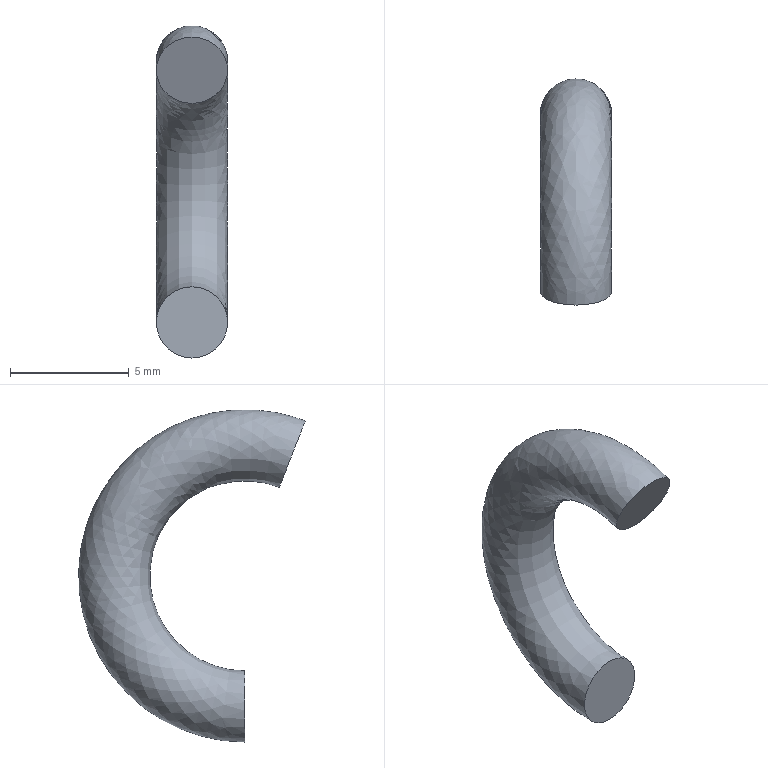Part | NX | features solid 2 | 1 solid | 3 faces | box 3 x 9.543 x 13.998 mm | volume 136.616 mm3 | plane 2 | spline 1
STEP:
#1=CARTESIAN_POINT('',(-1551.,413.545,19.726));
#2=VERTEX_POINT('',#1);
#3=CARTESIAN_POINT('',(-1551.,413.,21.123));
#4=DIRECTION('',(0.,-0.9315,-0.3636));
#5=DIRECTION('',(0.,0.3636,-0.9315));
#6=AXIS2_PLACEMENT_3D('',#3,#4,#5);
#7=CIRCLE('',#6,1.5);
#8=EDGE_CURVE('',#2,#2,#7,.T.);
#9=ORIENTED_EDGE('',*,*,#8,.T.);
#10=EDGE_LOOP('',(#9));
#11=FACE_BOUND('',#10,.T.);
#12=CARTESIAN_POINT('',(-1551.,413.,21.123));
#13=DIRECTION('',(0.,-0.9315,-0.3636));
#14=DIRECTION('',(0.,0.3636,-0.9315));
#15=AXIS2_PLACEMENT_3D('',#12,#13,#14);
#16=PLANE('',#15);
#17=ADVANCED_FACE('',(#11),#16,.T.);
#18=CARTESIAN_POINT('',(-1551.,415.,9.));
#19=VERTEX_POINT('',#18);
#20=CARTESIAN_POINT('',(-1551.,415.,10.5));
#21=DIRECTION('',(0.,-1.,0.));
#22=DIRECTION('',(0.,0.,-1.));
#23=AXIS2_PLACEMENT_3D('',#20,#21,#22);
#24=CIRCLE('',#23,1.5);
#25=EDGE_CURVE('',#19,#19,#24,.T.);
#26=ORIENTED_EDGE('',*,*,#25,.T.);
#27=EDGE_LOOP('',(#26));
#28=FACE_BOUND('',#27,.T.);
#29=CARTESIAN_POINT('',(-1551.,415.,10.5));
#30=DIRECTION('',(0.,-1.,0.));
#31=DIRECTION('',(0.,0.,-1.));
#32=AXIS2_PLACEMENT_3D('',#29,#30,#31);
#33=PLANE('',#32);
#34=ADVANCED_FACE('',(#28),#33,.T.);
#35=ORIENTED_EDGE('',*,*,#25,.F.);
#36=EDGE_LOOP('',(#35));
#37=FACE_BOUND('',#36,.T.);
#38=ORIENTED_EDGE('',*,*,#8,.F.);
#39=EDGE_LOOP('',(#38));
#40=FACE_BOUND('',#39,.T.);
#41=CARTESIAN_POINT('',(-1549.5,415.,9.97));
#42=CARTESIAN_POINT('',(-1549.5,416.255,9.958));
#43=CARTESIAN_POINT('',(-1549.5,417.618,10.391));
#44=CARTESIAN_POINT('',(-1549.5,419.793,12.094));
#45=CARTESIAN_POINT('',(-1549.5,420.5,13.222));
#46=CARTESIAN_POINT('',(-1549.5,421.165,15.703));
#47=CARTESIAN_POINT('',(-1549.5,421.079,17.179));
#48=CARTESIAN_POINT('',(-1549.5,420.163,19.234));
#49=CARTESIAN_POINT('',(-1549.5,419.645,19.935));
#50=CARTESIAN_POINT('',(-1549.5,418.39,21.062));
#51=CARTESIAN_POINT('',(-1549.5,416.38,22.219));
#52=CARTESIAN_POINT('',(-1549.5,413.962,22.092));
#53=CARTESIAN_POINT('',(-1549.5,412.807,21.617));
#54=CARTESIAN_POINT('',(-1549.5,415.,11.03));
#55=CARTESIAN_POINT('',(-1549.5,416.034,11.02));
#56=CARTESIAN_POINT('',(-1549.5,417.157,11.378));
#57=CARTESIAN_POINT('',(-1549.5,418.95,12.781));
#58=CARTESIAN_POINT('',(-1549.5,419.533,13.711));
#59=CARTESIAN_POINT('',(-1549.5,420.081,15.755));
#60=CARTESIAN_POINT('',(-1549.5,420.01,16.971));
#61=CARTESIAN_POINT('',(-1549.5,419.255,18.665));
#62=CARTESIAN_POINT('',(-1549.5,418.828,19.243));
#63=CARTESIAN_POINT('',(-1549.5,417.794,20.172));
#64=CARTESIAN_POINT('',(-1549.5,416.138,21.125));
#65=CARTESIAN_POINT('',(-1549.5,414.144,21.02));
#66=CARTESIAN_POINT('',(-1549.5,413.193,20.629));
#67=CARTESIAN_POINT('',(-1549.765,415.,11.735));
#68=CARTESIAN_POINT('',(-1549.765,415.888,11.726));
#69=CARTESIAN_POINT('',(-1549.765,416.851,12.033));
#70=CARTESIAN_POINT('',(-1549.765,418.39,13.237));
#71=CARTESIAN_POINT('',(-1549.765,418.89,14.035));
#72=CARTESIAN_POINT('',(-1549.765,419.36,15.79));
#73=CARTESIAN_POINT('',(-1549.765,419.3,16.834));
#74=CARTESIAN_POINT('',(-1549.765,418.652,18.288));
#75=CARTESIAN_POINT('',(-1549.765,418.285,18.783));
#76=CARTESIAN_POINT('',(-1549.765,417.398,19.58));
#77=CARTESIAN_POINT('',(-1549.765,415.976,20.398));
#78=CARTESIAN_POINT('',(-1549.765,414.266,20.308));
#79=CARTESIAN_POINT('',(-1549.765,413.449,19.973));
#80=CARTESIAN_POINT('',(-1550.47,415.,12.));
#81=CARTESIAN_POINT('',(-1550.47,415.833,11.992));
#82=CARTESIAN_POINT('',(-1550.47,416.736,12.28));
#83=CARTESIAN_POINT('',(-1550.47,418.179,13.409));
#84=CARTESIAN_POINT('',(-1550.47,418.648,14.158));
#85=CARTESIAN_POINT('',(-1550.47,419.089,15.803));
#86=CARTESIAN_POINT('',(-1550.47,419.032,16.782));
#87=CARTESIAN_POINT('',(-1550.47,418.425,18.145));
#88=CARTESIAN_POINT('',(-1550.47,418.081,18.61));
#89=CARTESIAN_POINT('',(-1550.47,417.249,19.358));
#90=CARTESIAN_POINT('',(-1550.47,415.916,20.125));
#91=CARTESIAN_POINT('',(-1550.47,414.311,20.041));
#92=CARTESIAN_POINT('',(-1550.47,413.545,19.726));
#93=CARTESIAN_POINT('',(-1551.53,415.,12.));
#94=CARTESIAN_POINT('',(-1551.53,415.833,11.992));
#95=CARTESIAN_POINT('',(-1551.53,416.736,12.28));
#96=CARTESIAN_POINT('',(-1551.53,418.179,13.409));
#97=CARTESIAN_POINT('',(-1551.53,418.648,14.158));
#98=CARTESIAN_POINT('',(-1551.53,419.089,15.803));
#99=CARTESIAN_POINT('',(-1551.53,419.032,16.782));
#100=CARTESIAN_POINT('',(-1551.53,418.425,18.145));
#101=CARTESIAN_POINT('',(-1551.53,418.081,18.61));
#102=CARTESIAN_POINT('',(-1551.53,417.249,19.358));
#103=CARTESIAN_POINT('',(-1551.53,415.916,20.125));
#104=CARTESIAN_POINT('',(-1551.53,414.311,20.041));
#105=CARTESIAN_POINT('',(-1551.53,413.545,19.726));
#106=CARTESIAN_POINT('',(-1552.235,415.,11.735));
#107=CARTESIAN_POINT('',(-1552.235,415.888,11.726));
#108=CARTESIAN_POINT('',(-1552.235,416.851,12.033));
#109=CARTESIAN_POINT('',(-1552.235,418.39,13.237));
#110=CARTESIAN_POINT('',(-1552.235,418.89,14.035));
#111=CARTESIAN_POINT('',(-1552.235,419.36,15.79));
#112=CARTESIAN_POINT('',(-1552.235,419.3,16.834));
#113=CARTESIAN_POINT('',(-1552.235,418.652,18.288));
#114=CARTESIAN_POINT('',(-1552.235,418.285,18.783));
#115=CARTESIAN_POINT('',(-1552.235,417.398,19.58));
#116=CARTESIAN_POINT('',(-1552.235,415.976,20.398));
#117=CARTESIAN_POINT('',(-1552.235,414.266,20.308));
#118=CARTESIAN_POINT('',(-1552.235,413.449,19.973));
#119=CARTESIAN_POINT('',(-1552.5,415.,11.03));
#120=CARTESIAN_POINT('',(-1552.5,416.034,11.02));
#121=CARTESIAN_POINT('',(-1552.5,417.157,11.378));
#122=CARTESIAN_POINT('',(-1552.5,418.95,12.781));
#123=CARTESIAN_POINT('',(-1552.5,419.533,13.711));
#124=CARTESIAN_POINT('',(-1552.5,420.081,15.755));
#125=CARTESIAN_POINT('',(-1552.5,420.01,16.971));
#126=CARTESIAN_POINT('',(-1552.5,419.255,18.665));
#127=CARTESIAN_POINT('',(-1552.5,418.828,19.243));
#128=CARTESIAN_POINT('',(-1552.5,417.794,20.172));
#129=CARTESIAN_POINT('',(-1552.5,416.138,21.125));
#130=CARTESIAN_POINT('',(-1552.5,414.144,21.02));
#131=CARTESIAN_POINT('',(-1552.5,413.193,20.629));
#132=CARTESIAN_POINT('',(-1552.5,415.,9.97));
#133=CARTESIAN_POINT('',(-1552.5,416.255,9.958));
#134=CARTESIAN_POINT('',(-1552.5,417.618,10.391));
#135=CARTESIAN_POINT('',(-1552.5,419.793,12.094));
#136=CARTESIAN_POINT('',(-1552.5,420.5,13.222));
#137=CARTESIAN_POINT('',(-1552.5,421.165,15.703));
#138=CARTESIAN_POINT('',(-1552.5,421.079,17.179));
#139=CARTESIAN_POINT('',(-1552.5,420.163,19.234));
#140=CARTESIAN_POINT('',(-1552.5,419.645,19.935));
#141=CARTESIAN_POINT('',(-1552.5,418.39,21.062));
#142=CARTESIAN_POINT('',(-1552.5,416.38,22.219));
#143=CARTESIAN_POINT('',(-1552.5,413.962,22.092));
#144=CARTESIAN_POINT('',(-1552.5,412.807,21.617));
#145=CARTESIAN_POINT('',(-1552.235,415.,9.265));
#146=CARTESIAN_POINT('',(-1552.235,416.402,9.252));
#147=CARTESIAN_POINT('',(-1552.235,417.923,9.736));
#148=CARTESIAN_POINT('',(-1552.235,420.353,11.638));
#149=CARTESIAN_POINT('',(-1552.235,421.143,12.898));
#150=CARTESIAN_POINT('',(-1552.235,421.885,15.668));
#151=CARTESIAN_POINT('',(-1552.235,421.789,17.317));
#152=CARTESIAN_POINT('',(-1552.235,420.767,19.612));
#153=CARTESIAN_POINT('',(-1552.235,420.188,20.395));
#154=CARTESIAN_POINT('',(-1552.235,418.786,21.653));
#155=CARTESIAN_POINT('',(-1552.235,416.542,22.945));
#156=CARTESIAN_POINT('',(-1552.235,413.84,22.803));
#157=CARTESIAN_POINT('',(-1552.235,412.551,22.274));
#158=CARTESIAN_POINT('',(-1551.53,415.,9.));
#159=CARTESIAN_POINT('',(-1551.53,416.457,8.986));
#160=CARTESIAN_POINT('',(-1551.53,418.038,9.49));
#161=CARTESIAN_POINT('',(-1551.53,420.564,11.466));
#162=CARTESIAN_POINT('',(-1551.53,421.384,12.776));
#163=CARTESIAN_POINT('',(-1551.53,422.156,15.655));
#164=CARTESIAN_POINT('',(-1551.53,422.056,17.368));
#165=CARTESIAN_POINT('',(-1551.53,420.994,19.754));
#166=CARTESIAN_POINT('',(-1551.53,420.392,20.568));
#167=CARTESIAN_POINT('',(-1551.53,418.935,21.876));
#168=CARTESIAN_POINT('',(-1551.53,416.602,23.218));
#169=CARTESIAN_POINT('',(-1551.53,413.795,23.071));
#170=CARTESIAN_POINT('',(-1551.53,412.455,22.521));
#171=CARTESIAN_POINT('',(-1550.47,415.,9.));
#172=CARTESIAN_POINT('',(-1550.47,416.457,8.986));
#173=CARTESIAN_POINT('',(-1550.47,418.038,9.49));
#174=CARTESIAN_POINT('',(-1550.47,420.564,11.466));
#175=CARTESIAN_POINT('',(-1550.47,421.384,12.776));
#176=CARTESIAN_POINT('',(-1550.47,422.156,15.655));
#177=CARTESIAN_POINT('',(-1550.47,422.056,17.368));
#178=CARTESIAN_POINT('',(-1550.47,420.994,19.754));
#179=CARTESIAN_POINT('',(-1550.47,420.392,20.568));
#180=CARTESIAN_POINT('',(-1550.47,418.935,21.876));
#181=CARTESIAN_POINT('',(-1550.47,416.602,23.218));
#182=CARTESIAN_POINT('',(-1550.47,413.795,23.071));
#183=CARTESIAN_POINT('',(-1550.47,412.455,22.521));
#184=CARTESIAN_POINT('',(-1549.765,415.,9.265));
#185=CARTESIAN_POINT('',(-1549.765,416.402,9.252));
#186=CARTESIAN_POINT('',(-1549.765,417.923,9.736));
#187=CARTESIAN_POINT('',(-1549.765,420.353,11.638));
#188=CARTESIAN_POINT('',(-1549.765,421.143,12.898));
#189=CARTESIAN_POINT('',(-1549.765,421.885,15.668));
#190=CARTESIAN_POINT('',(-1549.765,421.789,17.317));
#191=CARTESIAN_POINT('',(-1549.765,420.767,19.612));
#192=CARTESIAN_POINT('',(-1549.765,420.188,20.395));
#193=CARTESIAN_POINT('',(-1549.765,418.786,21.653));
#194=CARTESIAN_POINT('',(-1549.765,416.542,22.945));
#195=CARTESIAN_POINT('',(-1549.765,413.84,22.803));
#196=CARTESIAN_POINT('',(-1549.765,412.551,22.274));
#197=CARTESIAN_POINT('',(-1549.5,415.,9.97));
#198=CARTESIAN_POINT('',(-1549.5,416.255,9.958));
#199=CARTESIAN_POINT('',(-1549.5,417.618,10.391));
#200=CARTESIAN_POINT('',(-1549.5,419.793,12.094));
#201=CARTESIAN_POINT('',(-1549.5,420.5,13.222));
#202=CARTESIAN_POINT('',(-1549.5,421.165,15.703));
#203=CARTESIAN_POINT('',(-1549.5,421.079,17.179));
#204=CARTESIAN_POINT('',(-1549.5,420.163,19.234));
#205=CARTESIAN_POINT('',(-1549.5,419.645,19.935));
#206=CARTESIAN_POINT('',(-1549.5,418.39,21.062));
#207=CARTESIAN_POINT('',(-1549.5,416.38,22.219));
#208=CARTESIAN_POINT('',(-1549.5,413.962,22.092));
#209=CARTESIAN_POINT('',(-1549.5,412.807,21.617));
#210=CARTESIAN_POINT('',(-1549.5,415.,11.03));
#211=CARTESIAN_POINT('',(-1549.5,416.034,11.02));
#212=CARTESIAN_POINT('',(-1549.5,417.157,11.378));
#213=CARTESIAN_POINT('',(-1549.5,418.95,12.781));
#214=CARTESIAN_POINT('',(-1549.5,419.533,13.711));
#215=CARTESIAN_POINT('',(-1549.5,420.081,15.755));
#216=CARTESIAN_POINT('',(-1549.5,420.01,16.971));
#217=CARTESIAN_POINT('',(-1549.5,419.255,18.665));
#218=CARTESIAN_POINT('',(-1549.5,418.828,19.243));
#219=CARTESIAN_POINT('',(-1549.5,417.794,20.172));
#220=CARTESIAN_POINT('',(-1549.5,416.138,21.125));
#221=CARTESIAN_POINT('',(-1549.5,414.144,21.02));
#222=CARTESIAN_POINT('',(-1549.5,413.193,20.629));
#223=(BOUNDED_SURFACE()B_SPLINE_SURFACE(4,3,((#41,#42,#43,#44,#45,#46,#47,#48,#49,#50,#51,#52,#53),(#54,#55,#56,#57,#58,#59,#60,#61,#62,#63,#64,#65,#66),(#67,#68,#69,#70,#71,#72,#73,#74,#75,#76,#77,#78,#79),(#80,#81,#82,#83,#84,#85,#86,#87,#88,#89,#90,#91,#92),(#93,#94,#95,#96,#97,#98,#99,#100,#101,#102,#103,#104,#105),(#106,#107,#108,#109,#110,#111,#112,#113,#114,#115,#116,#117,#118),(#119,#120,#121,#122,#123,#124,#125,#126,#127,#128,#129,#130,#131),(#132,#133,#134,#135,#136,#137,#138,#139,#140,#141,#142,#143,#144),(#145,#146,#147,#148,#149,#150,#151,#152,#153,#154,#155,#156,#157),(#158,#159,#160,#161,#162,#163,#164,#165,#166,#167,#168,#169,#170),(#171,#172,#173,#174,#175,#176,#177,#178,#179,#180,#181,#182,#183),(#184,#185,#186,#187,#188,#189,#190,#191,#192,#193,#194,#195,#196),(#197,#198,#199,#200,#201,#202,#203,#204,#205,#206,#207,#208,#209),(#210,#211,#212,#213,#214,#215,#216,#217,#218,#219,#220,#221,#222)),.UNSPECIFIED.,.T.,.F.,.F.)B_SPLINE_SURFACE_WITH_KNOTS((2,3,3,3,3,3,2),(4,2,2,2,2,1,4),(-0.25,0.,0.25,0.5,0.75,1.,1.25),(0.,0.1875,0.375,0.5625,0.6875,0.8125,1.),.UNSPECIFIED.)GEOMETRIC_REPRESENTATION_ITEM()RATIONAL_B_SPLINE_SURFACE(((1.017,1.017,1.017,1.017,1.017,1.017,1.017,1.017,1.017,1.017,1.017,1.017,1.017),(1.017,1.017,1.017,1.017,1.017,1.017,1.017,1.017,1.017,1.017,1.017,1.017,1.017),(0.9585,0.9585,0.9585,0.9585,0.9585,0.9585,0.9585,0.9585,0.9585,0.9585,0.9585,0.9585,0.9585),(1.017,1.017,1.017,1.017,1.017,1.017,1.017,1.017,1.017,1.017,1.017,1.017,1.017),(1.017,1.017,1.017,1.017,1.017,1.017,1.017,1.017,1.017,1.017,1.017,1.017,1.017),(0.9585,0.9585,0.9585,0.9585,0.9585,0.9585,0.9585,0.9585,0.9585,0.9585,0.9585,0.9585,0.9585),(1.017,1.017,1.017,1.017,1.017,1.017,1.017,1.017,1.017,1.017,1.017,1.017,1.017),(1.017,1.017,1.017,1.017,1.017,1.017,1.017,1.017,1.017,1.017,1.017,1.017,1.017),(0.9585,0.9585,0.9585,0.9585,0.9585,0.9585,0.9585,0.9585,0.9585,0.9585,0.9585,0.9585,0.9585),(1.017,1.017,1.017,1.017,1.017,1.017,1.017,1.017,1.017,1.017,1.017,1.017,1.017),(1.017,1.017,1.017,1.017,1.017,1.017,1.017,1.017,1.017,1.017,1.017,1.017,1.017),(0.9585,0.9585,0.9585,0.9585,0.9585,0.9585,0.9585,0.9585,0.9585,0.9585,0.9585,0.9585,0.9585),(1.017,1.017,1.017,1.017,1.017,1.017,1.017,1.017,1.017,1.017,1.017,1.017,1.017),(1.017,1.017,1.017,1.017,1.017,1.017,1.017,1.017,1.017,1.017,1.017,1.017,1.017)))REPRESENTATION_ITEM('')SURFACE());
#224=ADVANCED_FACE('',(#37,#40),#223,.F.);
#225=CLOSED_SHELL('',(#17,#34,#224));
#226=MANIFOLD_SOLID_BREP('',#225);
#227=(LENGTH_UNIT()NAMED_UNIT(*)SI_UNIT(.MILLI.,.METRE.));
#228=UNCERTAINTY_MEASURE_WITH_UNIT(LENGTH_MEASURE(0.00001),#227,'','');
#229=(NAMED_UNIT(*)PLANE_ANGLE_UNIT()SI_UNIT($,.RADIAN.));
#230=(NAMED_UNIT(*)SI_UNIT($,.STERADIAN.)SOLID_ANGLE_UNIT());
#231=(GEOMETRIC_REPRESENTATION_CONTEXT(3)GLOBAL_UNCERTAINTY_ASSIGNED_CONTEXT((#228))GLOBAL_UNIT_ASSIGNED_CONTEXT((#227,#229,#230))REPRESENTATION_CONTEXT('',''));
#232=ADVANCED_BREP_SHAPE_REPRESENTATION('',(#226),#231);